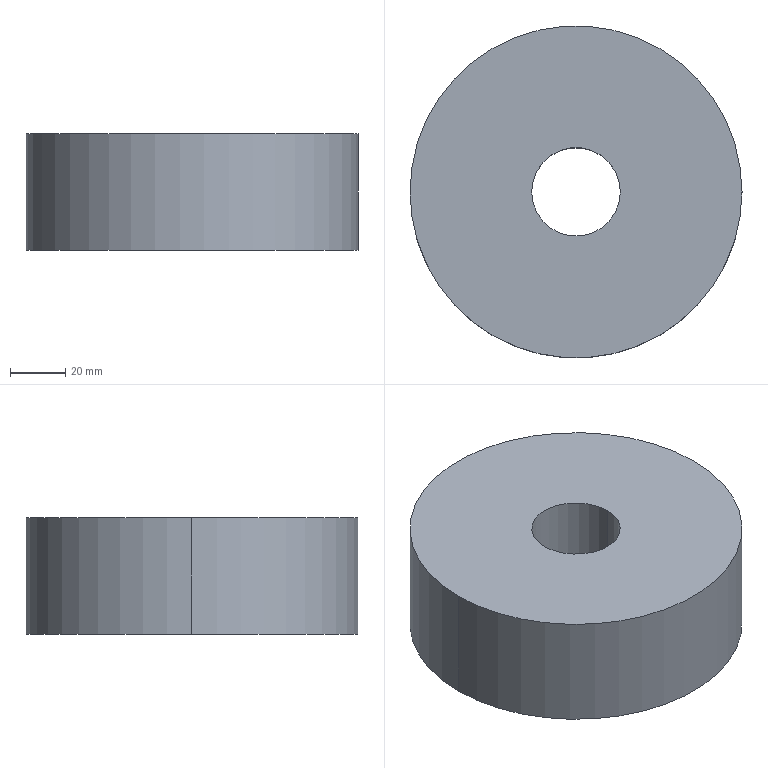Part | STEP file | 10000020487swp000-1 | 1 solid | 6 faces | box 120 x 120 x 42 mm | volume 441230 mm3 | cylinder 4 | plane 2 | commonest cylinder face diameters 32 x2 120 x2
STEP:
#1=CARTESIAN_POINT('',(-16.,0.,21.));
#2=VERTEX_POINT('',#1);
#3=CARTESIAN_POINT('',(16.,0.,21.));
#4=VERTEX_POINT('',#3);
#5=CARTESIAN_POINT('',(0.,0.,21.));
#6=DIRECTION('',(0.,0.,1.));
#7=DIRECTION('',(1.,0.,0.));
#8=AXIS2_PLACEMENT_3D('',#5,#6,#7);
#9=CIRCLE('',#8,16.);
#10=EDGE_CURVE('',#2,#4,#9,.T.);
#11=ORIENTED_EDGE('',*,*,#10,.T.);
#12=CARTESIAN_POINT('',(16.,0.,-21.));
#13=VERTEX_POINT('',#12);
#14=CARTESIAN_POINT('',(16.,0.,21.));
#15=DIRECTION('',(0.,0.,-1.));
#16=VECTOR('',#15,1000.);
#17=LINE('',#14,#16);
#18=EDGE_CURVE('',#4,#13,#17,.T.);
#19=ORIENTED_EDGE('',*,*,#18,.T.);
#20=CARTESIAN_POINT('',(-16.,0.,-21.));
#21=VERTEX_POINT('',#20);
#22=CARTESIAN_POINT('',(0.,0.,-21.));
#23=DIRECTION('',(0.,0.,1.));
#24=DIRECTION('',(1.,0.,0.));
#25=AXIS2_PLACEMENT_3D('',#22,#23,#24);
#26=CIRCLE('',#25,16.);
#27=EDGE_CURVE('',#21,#13,#26,.T.);
#28=ORIENTED_EDGE('',*,*,#27,.F.);
#29=CARTESIAN_POINT('',(-16.,0.,21.));
#30=DIRECTION('',(0.,0.,-1.));
#31=VECTOR('',#30,1000.);
#32=LINE('',#29,#31);
#33=EDGE_CURVE('',#2,#21,#32,.T.);
#34=ORIENTED_EDGE('',*,*,#33,.F.);
#35=EDGE_LOOP('',(#11,#19,#28,#34));
#36=FACE_OUTER_BOUND('',#35,.T.);
#37=CARTESIAN_POINT('',(0.,0.,21.));
#38=DIRECTION('',(0.,0.,-1.));
#39=DIRECTION('',(-1.,0.,0.));
#40=AXIS2_PLACEMENT_3D('',#37,#38,#39);
#41=CYLINDRICAL_SURFACE('',#40,16.);
#42=ADVANCED_FACE('',(#36),#41,.F.);
#43=CARTESIAN_POINT('',(60.,0.,21.));
#44=VERTEX_POINT('',#43);
#45=CARTESIAN_POINT('',(-60.,0.,21.));
#46=VERTEX_POINT('',#45);
#47=CARTESIAN_POINT('',(0.,0.,21.));
#48=DIRECTION('',(0.,0.,1.));
#49=DIRECTION('',(1.,0.,0.));
#50=AXIS2_PLACEMENT_3D('',#47,#48,#49);
#51=CIRCLE('',#50,60.);
#52=EDGE_CURVE('',#44,#46,#51,.T.);
#53=ORIENTED_EDGE('',*,*,#52,.F.);
#54=CARTESIAN_POINT('',(60.,0.,-21.));
#55=VERTEX_POINT('',#54);
#56=CARTESIAN_POINT('',(60.,0.,21.));
#57=DIRECTION('',(0.,0.,-1.));
#58=VECTOR('',#57,1000.);
#59=LINE('',#56,#58);
#60=EDGE_CURVE('',#44,#55,#59,.T.);
#61=ORIENTED_EDGE('',*,*,#60,.T.);
#62=CARTESIAN_POINT('',(-60.,0.,-21.));
#63=VERTEX_POINT('',#62);
#64=CARTESIAN_POINT('',(0.,0.,-21.));
#65=DIRECTION('',(0.,0.,1.));
#66=DIRECTION('',(1.,0.,0.));
#67=AXIS2_PLACEMENT_3D('',#64,#65,#66);
#68=CIRCLE('',#67,60.);
#69=EDGE_CURVE('',#55,#63,#68,.T.);
#70=ORIENTED_EDGE('',*,*,#69,.T.);
#71=CARTESIAN_POINT('',(-60.,0.,21.));
#72=DIRECTION('',(0.,0.,-1.));
#73=VECTOR('',#72,1000.);
#74=LINE('',#71,#73);
#75=EDGE_CURVE('',#46,#63,#74,.T.);
#76=ORIENTED_EDGE('',*,*,#75,.F.);
#77=EDGE_LOOP('',(#53,#61,#70,#76));
#78=FACE_OUTER_BOUND('',#77,.T.);
#79=CARTESIAN_POINT('',(0.,0.,21.));
#80=DIRECTION('',(0.,0.,-1.));
#81=DIRECTION('',(-1.,0.,0.));
#82=AXIS2_PLACEMENT_3D('',#79,#80,#81);
#83=CYLINDRICAL_SURFACE('',#82,60.);
#84=ADVANCED_FACE('',(#78),#83,.T.);
#85=CARTESIAN_POINT('',(0.,0.,21.));
#86=DIRECTION('',(0.,0.,1.));
#87=DIRECTION('',(1.,0.,0.));
#88=AXIS2_PLACEMENT_3D('',#85,#86,#87);
#89=CIRCLE('',#88,60.);
#90=EDGE_CURVE('',#46,#44,#89,.T.);
#91=ORIENTED_EDGE('',*,*,#90,.T.);
#92=ORIENTED_EDGE('',*,*,#52,.T.);
#93=EDGE_LOOP('',(#91,#92));
#94=FACE_OUTER_BOUND('',#93,.T.);
#95=ORIENTED_EDGE('',*,*,#10,.F.);
#96=CARTESIAN_POINT('',(0.,0.,21.));
#97=DIRECTION('',(0.,0.,1.));
#98=DIRECTION('',(1.,0.,0.));
#99=AXIS2_PLACEMENT_3D('',#96,#97,#98);
#100=CIRCLE('',#99,16.);
#101=EDGE_CURVE('',#4,#2,#100,.T.);
#102=ORIENTED_EDGE('',*,*,#101,.F.);
#103=EDGE_LOOP('',(#95,#102));
#104=FACE_BOUND('',#103,.T.);
#105=CARTESIAN_POINT('',(0.,0.,21.));
#106=DIRECTION('',(0.,0.,1.));
#107=DIRECTION('',(1.,0.,0.));
#108=AXIS2_PLACEMENT_3D('',#105,#106,#107);
#109=PLANE('',#108);
#110=ADVANCED_FACE('',(#94,#104),#109,.T.);
#111=CARTESIAN_POINT('',(0.,0.,-21.));
#112=DIRECTION('',(0.,0.,1.));
#113=DIRECTION('',(1.,0.,0.));
#114=AXIS2_PLACEMENT_3D('',#111,#112,#113);
#115=CIRCLE('',#114,60.);
#116=EDGE_CURVE('',#63,#55,#115,.T.);
#117=ORIENTED_EDGE('',*,*,#116,.F.);
#118=ORIENTED_EDGE('',*,*,#69,.F.);
#119=EDGE_LOOP('',(#117,#118));
#120=FACE_OUTER_BOUND('',#119,.T.);
#121=ORIENTED_EDGE('',*,*,#27,.T.);
#122=CARTESIAN_POINT('',(0.,0.,-21.));
#123=DIRECTION('',(0.,0.,1.));
#124=DIRECTION('',(1.,0.,0.));
#125=AXIS2_PLACEMENT_3D('',#122,#123,#124);
#126=CIRCLE('',#125,16.);
#127=EDGE_CURVE('',#13,#21,#126,.T.);
#128=ORIENTED_EDGE('',*,*,#127,.T.);
#129=EDGE_LOOP('',(#121,#128));
#130=FACE_BOUND('',#129,.T.);
#131=CARTESIAN_POINT('',(0.,0.,-21.));
#132=DIRECTION('',(0.,0.,1.));
#133=DIRECTION('',(1.,0.,0.));
#134=AXIS2_PLACEMENT_3D('',#131,#132,#133);
#135=PLANE('',#134);
#136=ADVANCED_FACE('',(#120,#130),#135,.F.);
#137=ORIENTED_EDGE('',*,*,#60,.F.);
#138=ORIENTED_EDGE('',*,*,#90,.F.);
#139=ORIENTED_EDGE('',*,*,#75,.T.);
#140=ORIENTED_EDGE('',*,*,#116,.T.);
#141=EDGE_LOOP('',(#137,#138,#139,#140));
#142=FACE_OUTER_BOUND('',#141,.T.);
#143=CARTESIAN_POINT('',(0.,0.,21.));
#144=DIRECTION('',(0.,0.,-1.));
#145=DIRECTION('',(-1.,0.,0.));
#146=AXIS2_PLACEMENT_3D('',#143,#144,#145);
#147=CYLINDRICAL_SURFACE('',#146,60.);
#148=ADVANCED_FACE('',(#142),#147,.T.);
#149=ORIENTED_EDGE('',*,*,#18,.F.);
#150=ORIENTED_EDGE('',*,*,#101,.T.);
#151=ORIENTED_EDGE('',*,*,#33,.T.);
#152=ORIENTED_EDGE('',*,*,#127,.F.);
#153=EDGE_LOOP('',(#149,#150,#151,#152));
#154=FACE_OUTER_BOUND('',#153,.T.);
#155=CARTESIAN_POINT('',(0.,0.,21.));
#156=DIRECTION('',(0.,0.,-1.));
#157=DIRECTION('',(-1.,0.,0.));
#158=AXIS2_PLACEMENT_3D('',#155,#156,#157);
#159=CYLINDRICAL_SURFACE('',#158,16.);
#160=ADVANCED_FACE('',(#154),#159,.F.);
#161=CLOSED_SHELL('',(#42,#84,#110,#136,#148,#160));
#162=MANIFOLD_SOLID_BREP('',#161);
#163=CARTESIAN_POINT('',(0.,0.,0.));
#164=DIRECTION('',(0.,0.,1.));
#165=DIRECTION('',(1.,0.,0.));
#166=AXIS2_PLACEMENT_3D('',#163,#164,#165);
#167=(LENGTH_UNIT()NAMED_UNIT(*)SI_UNIT(.MILLI.,.METRE.));
#168=UNCERTAINTY_MEASURE_WITH_UNIT(LENGTH_MEASURE(0.00001),#167,'','');
#169=(NAMED_UNIT(*)PLANE_ANGLE_UNIT()SI_UNIT($,.RADIAN.));
#170=(NAMED_UNIT(*)SI_UNIT($,.STERADIAN.)SOLID_ANGLE_UNIT());
#171=(GEOMETRIC_REPRESENTATION_CONTEXT(3)GLOBAL_UNCERTAINTY_ASSIGNED_CONTEXT((#168))GLOBAL_UNIT_ASSIGNED_CONTEXT((#167,#169,#170))REPRESENTATION_CONTEXT('',''));
#172=ADVANCED_BREP_SHAPE_REPRESENTATION('',(#162,#166),#171);